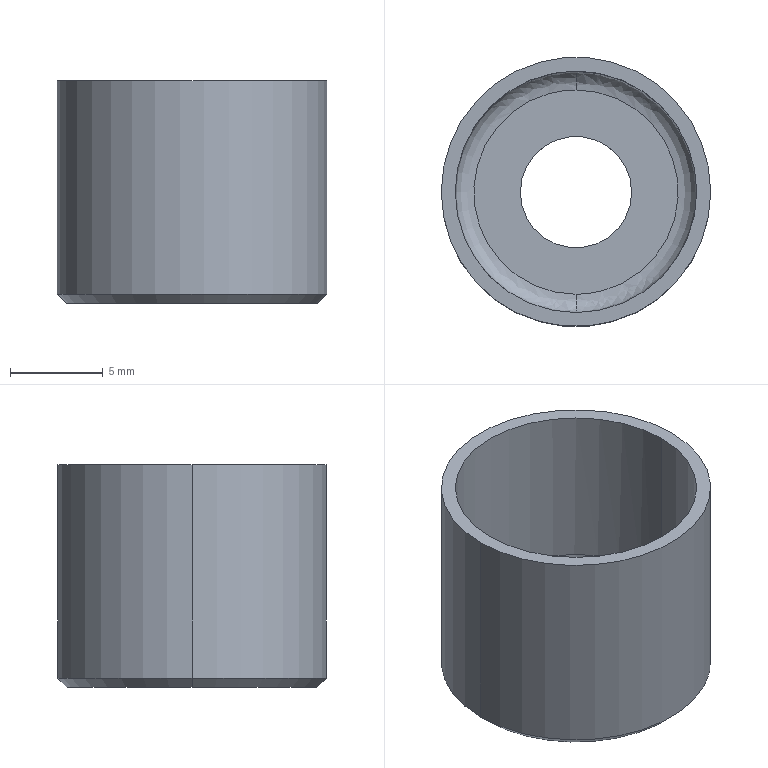Part | SolidWorks | features BaseBody 1 | 1 solid | 13 faces | box 14.5 x 14.5 x 12 mm | volume 600.582 mm3 | cylinder 6 | plane 3 | spline 2 | cone 2 | commonest cylinder face diameters 6 x2 13 x2 14.5 x2
STEP:
#1=CARTESIAN_POINT('',(480.537,43.215,-64.134));
#2=VERTEX_POINT('',#1);
#3=CARTESIAN_POINT('',(480.537,32.215,-64.134));
#4=VERTEX_POINT('',#3);
#5=CARTESIAN_POINT('',(480.537,43.215,-64.134));
#6=CARTESIAN_POINT('',(491.537,43.215,-64.134));
#7=CARTESIAN_POINT('',(491.537,32.215,-64.134));
#8=CARTESIAN_POINT('',(480.537,32.215,-64.134));
#9=(BOUNDED_CURVE()B_SPLINE_CURVE(3,(#5,#6,#7,#8),.UNSPECIFIED.,.F.,.F.)B_SPLINE_CURVE_WITH_KNOTS((4,4),(0.,1.),.UNSPECIFIED.)CURVE()GEOMETRIC_REPRESENTATION_ITEM()RATIONAL_B_SPLINE_CURVE((1.,0.3333,0.3333,1.))REPRESENTATION_ITEM(''));
#10=EDGE_CURVE('',#2,#4,#9,.T.);
#11=ORIENTED_EDGE('',*,*,#10,.T.);
#12=CARTESIAN_POINT('',(480.537,31.215,-63.134));
#13=VERTEX_POINT('',#12);
#14=CARTESIAN_POINT('',(480.537,32.215,-64.134));
#15=CARTESIAN_POINT('',(480.537,32.089,-64.134));
#16=CARTESIAN_POINT('',(480.537,31.827,-64.084));
#17=CARTESIAN_POINT('',(480.537,31.488,-63.861));
#18=CARTESIAN_POINT('',(480.537,31.265,-63.521));
#19=CARTESIAN_POINT('',(480.537,31.215,-63.26));
#20=CARTESIAN_POINT('',(480.537,31.215,-63.134));
#21=B_SPLINE_CURVE_WITH_KNOTS('',3,(#14,#15,#16,#17,#18,#19,#20),.UNSPECIFIED.,.F.,.F.,(4,1,1,1,4),(0.01923,0.25,0.5,0.75,0.9808),.UNSPECIFIED.);
#22=EDGE_CURVE('',#4,#13,#21,.T.);
#23=ORIENTED_EDGE('',*,*,#22,.T.);
#24=CARTESIAN_POINT('',(487.037,37.715,-63.134));
#25=VERTEX_POINT('',#24);
#26=CARTESIAN_POINT('',(487.037,37.715,-63.134));
#27=CARTESIAN_POINT('',(487.037,36.864,-63.134));
#28=CARTESIAN_POINT('',(486.868,36.013,-63.134));
#29=CARTESIAN_POINT('',(486.216,34.441,-63.134));
#30=CARTESIAN_POINT('',(485.735,33.72,-63.134));
#31=CARTESIAN_POINT('',(484.531,32.517,-63.134));
#32=CARTESIAN_POINT('',(483.81,32.035,-63.134));
#33=CARTESIAN_POINT('',(482.238,31.384,-63.134));
#34=CARTESIAN_POINT('',(481.388,31.215,-63.134));
#35=CARTESIAN_POINT('',(480.537,31.215,-63.134));
#36=B_SPLINE_CURVE_WITH_KNOTS('',3,(#26,#27,#28,#29,#30,#31,#32,#33,#34,#35),.UNSPECIFIED.,.F.,.F.,(4,2,2,2,4),(0.5,0.625,0.75,0.875,1.),.UNSPECIFIED.);
#37=EDGE_CURVE('',#25,#13,#36,.T.);
#38=ORIENTED_EDGE('',*,*,#37,.F.);
#39=CARTESIAN_POINT('',(480.537,44.215,-63.134));
#40=VERTEX_POINT('',#39);
#41=CARTESIAN_POINT('',(480.537,44.215,-63.134));
#42=CARTESIAN_POINT('',(481.388,44.215,-63.134));
#43=CARTESIAN_POINT('',(482.238,44.046,-63.134));
#44=CARTESIAN_POINT('',(483.81,43.394,-63.134));
#45=CARTESIAN_POINT('',(484.531,42.913,-63.134));
#46=CARTESIAN_POINT('',(485.735,41.709,-63.134));
#47=CARTESIAN_POINT('',(486.216,40.988,-63.134));
#48=CARTESIAN_POINT('',(486.868,39.416,-63.134));
#49=CARTESIAN_POINT('',(487.037,38.566,-63.134));
#50=CARTESIAN_POINT('',(487.037,37.715,-63.134));
#51=B_SPLINE_CURVE_WITH_KNOTS('',3,(#41,#42,#43,#44,#45,#46,#47,#48,#49,#50),.UNSPECIFIED.,.F.,.F.,(4,2,2,2,4),(0.,0.125,0.25,0.375,0.5),.UNSPECIFIED.);
#52=EDGE_CURVE('',#40,#25,#51,.T.);
#53=ORIENTED_EDGE('',*,*,#52,.F.);
#54=CARTESIAN_POINT('',(480.537,43.215,-64.134));
#55=CARTESIAN_POINT('',(480.537,43.34,-64.134));
#56=CARTESIAN_POINT('',(480.537,43.602,-64.084));
#57=CARTESIAN_POINT('',(480.537,43.942,-63.861));
#58=CARTESIAN_POINT('',(480.537,44.165,-63.521));
#59=CARTESIAN_POINT('',(480.537,44.215,-63.26));
#60=CARTESIAN_POINT('',(480.537,44.215,-63.134));
#61=B_SPLINE_CURVE_WITH_KNOTS('',3,(#54,#55,#56,#57,#58,#59,#60),.UNSPECIFIED.,.F.,.F.,(4,1,1,1,4),(0.01923,0.25,0.5,0.75,0.9808),.UNSPECIFIED.);
#62=EDGE_CURVE('',#2,#40,#61,.T.);
#63=ORIENTED_EDGE('',*,*,#62,.F.);
#64=EDGE_LOOP('',(#11,#23,#38,#53,#63));
#65=FACE_OUTER_BOUND('',#64,.T.);
#66=CARTESIAN_POINT('',(480.537,32.215,-64.134));
#67=CARTESIAN_POINT('',(491.537,32.215,-64.134));
#68=CARTESIAN_POINT('',(491.537,43.215,-64.134));
#69=CARTESIAN_POINT('',(480.537,43.215,-64.134));
#70=CARTESIAN_POINT('',(480.537,32.089,-64.134));
#71=CARTESIAN_POINT('',(491.788,32.089,-64.134));
#72=CARTESIAN_POINT('',(491.788,43.34,-64.134));
#73=CARTESIAN_POINT('',(480.537,43.34,-64.134));
#74=CARTESIAN_POINT('',(480.537,31.827,-64.084));
#75=CARTESIAN_POINT('',(492.312,31.827,-64.084));
#76=CARTESIAN_POINT('',(492.312,43.602,-64.084));
#77=CARTESIAN_POINT('',(480.537,43.602,-64.084));
#78=CARTESIAN_POINT('',(480.537,31.488,-63.861));
#79=CARTESIAN_POINT('',(492.991,31.488,-63.861));
#80=CARTESIAN_POINT('',(492.991,43.942,-63.861));
#81=CARTESIAN_POINT('',(480.537,43.942,-63.861));
#82=CARTESIAN_POINT('',(480.537,31.265,-63.521));
#83=CARTESIAN_POINT('',(493.437,31.265,-63.521));
#84=CARTESIAN_POINT('',(493.437,44.165,-63.521));
#85=CARTESIAN_POINT('',(480.537,44.165,-63.521));
#86=CARTESIAN_POINT('',(480.537,31.215,-63.26));
#87=CARTESIAN_POINT('',(493.537,31.215,-63.26));
#88=CARTESIAN_POINT('',(493.537,44.215,-63.26));
#89=CARTESIAN_POINT('',(480.537,44.215,-63.26));
#90=CARTESIAN_POINT('',(480.537,31.215,-63.134));
#91=CARTESIAN_POINT('',(493.537,31.215,-63.134));
#92=CARTESIAN_POINT('',(493.537,44.215,-63.134));
#93=CARTESIAN_POINT('',(480.537,44.215,-63.134));
#94=(BOUNDED_SURFACE()B_SPLINE_SURFACE(3,3,((#66,#67,#68,#69),(#70,#71,#72,#73),(#74,#75,#76,#77),(#78,#79,#80,#81),(#82,#83,#84,#85),(#86,#87,#88,#89),(#90,#91,#92,#93)),.UNSPECIFIED.,.F.,.F.,.F.)B_SPLINE_SURFACE_WITH_KNOTS((4,1,1,1,4),(4,4),(0.01923,0.25,0.5,0.75,0.9808),(0.,1.),.UNSPECIFIED.)GEOMETRIC_REPRESENTATION_ITEM()RATIONAL_B_SPLINE_SURFACE(((1.,0.3333,0.3333,1.),(1.,0.3333,0.3333,1.),(1.,0.3333,0.3333,1.),(1.,0.3333,0.3333,1.),(1.,0.3333,0.3333,1.),(1.,0.3333,0.3333,1.),(1.,0.3333,0.3333,1.)))REPRESENTATION_ITEM('')SURFACE());
#95=ADVANCED_FACE('',(#65),#94,.T.);
#96=CARTESIAN_POINT('',(473.287,37.715,-65.634));
#97=VERTEX_POINT('',#96);
#98=CARTESIAN_POINT('',(487.787,37.715,-65.634));
#99=VERTEX_POINT('',#98);
#100=CARTESIAN_POINT('',(480.537,37.715,-65.634));
#101=DIRECTION('',(0.000000013,0.,-1.));
#102=DIRECTION('',(0.,1.,0.));
#103=AXIS2_PLACEMENT_3D('',#100,#101,#102);
#104=CIRCLE('',#103,7.25);
#105=EDGE_CURVE('',#97,#99,#104,.T.);
#106=ORIENTED_EDGE('',*,*,#105,.F.);
#107=CARTESIAN_POINT('',(473.287,37.715,-54.134));
#108=VERTEX_POINT('',#107);
#109=CARTESIAN_POINT('',(473.287,37.715,-65.634));
#110=DIRECTION('',(-0.000000013,0.,1.));
#111=VECTOR('',#110,1000.);
#112=LINE('',#109,#111);
#113=EDGE_CURVE('',#97,#108,#112,.T.);
#114=ORIENTED_EDGE('',*,*,#113,.T.);
#115=CARTESIAN_POINT('',(487.787,37.715,-54.134));
#116=VERTEX_POINT('',#115);
#117=CARTESIAN_POINT('',(480.537,37.715,-54.134));
#118=DIRECTION('',(-0.000000013,0.,1.));
#119=DIRECTION('',(1.,0.,0.000000013));
#120=AXIS2_PLACEMENT_3D('',#117,#118,#119);
#121=CIRCLE('',#120,7.25);
#122=EDGE_CURVE('',#116,#108,#121,.T.);
#123=ORIENTED_EDGE('',*,*,#122,.F.);
#124=CARTESIAN_POINT('',(487.787,37.715,-65.634));
#125=DIRECTION('',(-0.000000013,0.,1.));
#126=VECTOR('',#125,1000.);
#127=LINE('',#124,#126);
#128=EDGE_CURVE('',#99,#116,#127,.T.);
#129=ORIENTED_EDGE('',*,*,#128,.F.);
#130=EDGE_LOOP('',(#106,#114,#123,#129));
#131=FACE_OUTER_BOUND('',#130,.T.);
#132=CARTESIAN_POINT('',(480.537,37.715,-65.634));
#133=DIRECTION('',(-0.000000013,0.,1.));
#134=DIRECTION('',(1.,0.,0.000000013));
#135=AXIS2_PLACEMENT_3D('',#132,#133,#134);
#136=CYLINDRICAL_SURFACE('',#135,7.25);
#137=ADVANCED_FACE('',(#131),#136,.T.);
#138=CARTESIAN_POINT('',(473.787,37.715,-66.134));
#139=VERTEX_POINT('',#138);
#140=CARTESIAN_POINT('',(487.287,37.715,-66.134));
#141=VERTEX_POINT('',#140);
#142=CARTESIAN_POINT('',(480.537,37.715,-66.134));
#143=DIRECTION('',(0.000000013,0.,-1.));
#144=DIRECTION('',(1.,0.,0.000000013));
#145=AXIS2_PLACEMENT_3D('',#142,#143,#144);
#146=CIRCLE('',#145,6.75);
#147=EDGE_CURVE('',#139,#141,#146,.T.);
#148=ORIENTED_EDGE('',*,*,#147,.F.);
#149=CARTESIAN_POINT('',(473.787,37.715,-66.134));
#150=DIRECTION('',(-0.7071,0.,0.7071));
#151=VECTOR('',#150,1000.);
#152=LINE('',#149,#151);
#153=EDGE_CURVE('',#139,#97,#152,.T.);
#154=ORIENTED_EDGE('',*,*,#153,.T.);
#155=ORIENTED_EDGE('',*,*,#105,.T.);
#156=CARTESIAN_POINT('',(487.287,37.715,-66.134));
#157=DIRECTION('',(0.7071,0.,0.7071));
#158=VECTOR('',#157,1000.);
#159=LINE('',#156,#158);
#160=EDGE_CURVE('',#141,#99,#159,.T.);
#161=ORIENTED_EDGE('',*,*,#160,.F.);
#162=EDGE_LOOP('',(#148,#154,#155,#161));
#163=FACE_OUTER_BOUND('',#162,.T.);
#164=CARTESIAN_POINT('',(480.537,37.715,-66.134));
#165=DIRECTION('',(-0.000000013,0.,1.));
#166=DIRECTION('',(1.,0.,0.000000013));
#167=AXIS2_PLACEMENT_3D('',#164,#165,#166);
#168=CONICAL_SURFACE('',#167,6.75,0.7854);
#169=ADVANCED_FACE('',(#163),#168,.T.);
#170=CARTESIAN_POINT('',(474.037,37.715,-63.134));
#171=VERTEX_POINT('',#170);
#172=CARTESIAN_POINT('',(480.537,31.215,-63.134));
#173=CARTESIAN_POINT('',(479.686,31.215,-63.134));
#174=CARTESIAN_POINT('',(478.835,31.384,-63.134));
#175=CARTESIAN_POINT('',(477.263,32.035,-63.134));
#176=CARTESIAN_POINT('',(476.542,32.517,-63.134));
#177=CARTESIAN_POINT('',(475.339,33.72,-63.134));
#178=CARTESIAN_POINT('',(474.857,34.441,-63.134));
#179=CARTESIAN_POINT('',(474.206,36.013,-63.134));
#180=CARTESIAN_POINT('',(474.037,36.864,-63.134));
#181=CARTESIAN_POINT('',(474.037,37.715,-63.134));
#182=B_SPLINE_CURVE_WITH_KNOTS('',3,(#172,#173,#174,#175,#176,#177,#178,#179,#180,#181),.UNSPECIFIED.,.F.,.F.,(4,2,2,2,4),(0.,0.125,0.25,0.375,0.5),.UNSPECIFIED.);
#183=EDGE_CURVE('',#13,#171,#182,.T.);
#184=ORIENTED_EDGE('',*,*,#183,.T.);
#185=CARTESIAN_POINT('',(474.037,37.715,-54.134));
#186=VERTEX_POINT('',#185);
#187=CARTESIAN_POINT('',(474.037,37.715,-63.134));
#188=DIRECTION('',(-0.000000013,0.,1.));
#189=VECTOR('',#188,1000.);
#190=LINE('',#187,#189);
#191=EDGE_CURVE('',#171,#186,#190,.T.);
#192=ORIENTED_EDGE('',*,*,#191,.T.);
#193=CARTESIAN_POINT('',(487.037,37.715,-54.134));
#194=VERTEX_POINT('',#193);
#195=CARTESIAN_POINT('',(480.537,37.715,-54.134));
#196=DIRECTION('',(0.000000013,0.,-1.));
#197=DIRECTION('',(1.,0.,0.000000013));
#198=AXIS2_PLACEMENT_3D('',#195,#196,#197);
#199=CIRCLE('',#198,6.5);
#200=EDGE_CURVE('',#194,#186,#199,.T.);
#201=ORIENTED_EDGE('',*,*,#200,.F.);
#202=CARTESIAN_POINT('',(487.037,37.715,-63.134));
#203=DIRECTION('',(-0.000000013,0.,1.));
#204=VECTOR('',#203,1000.);
#205=LINE('',#202,#204);
#206=EDGE_CURVE('',#25,#194,#205,.T.);
#207=ORIENTED_EDGE('',*,*,#206,.F.);
#208=ORIENTED_EDGE('',*,*,#37,.T.);
#209=EDGE_LOOP('',(#184,#192,#201,#207,#208));
#210=FACE_OUTER_BOUND('',#209,.T.);
#211=CARTESIAN_POINT('',(480.537,37.715,-63.134));
#212=DIRECTION('',(-0.000000013,0.,1.));
#213=DIRECTION('',(1.,0.,0.000000013));
#214=AXIS2_PLACEMENT_3D('',#211,#212,#213);
#215=CYLINDRICAL_SURFACE('',#214,6.5);
#216=ADVANCED_FACE('',(#210),#215,.F.);
#217=CARTESIAN_POINT('',(483.537,37.715,-66.134));
#218=VERTEX_POINT('',#217);
#219=CARTESIAN_POINT('',(477.537,37.715,-66.134));
#220=VERTEX_POINT('',#219);
#221=CARTESIAN_POINT('',(480.537,37.715,-66.134));
#222=DIRECTION('',(0.000000013,0.,-1.));
#223=DIRECTION('',(1.,0.,0.000000013));
#224=AXIS2_PLACEMENT_3D('',#221,#222,#223);
#225=CIRCLE('',#224,3.);
#226=EDGE_CURVE('',#218,#220,#225,.T.);
#227=ORIENTED_EDGE('',*,*,#226,.T.);
#228=CARTESIAN_POINT('',(477.537,37.715,-64.134));
#229=VERTEX_POINT('',#228);
#230=CARTESIAN_POINT('',(477.537,37.715,-66.134));
#231=DIRECTION('',(-0.000000013,0.,1.));
#232=VECTOR('',#231,1000.);
#233=LINE('',#230,#232);
#234=EDGE_CURVE('',#220,#229,#233,.T.);
#235=ORIENTED_EDGE('',*,*,#234,.T.);
#236=CARTESIAN_POINT('',(483.537,37.715,-64.134));
#237=VERTEX_POINT('',#236);
#238=CARTESIAN_POINT('',(480.537,37.715,-64.134));
#239=DIRECTION('',(-0.000000013,0.,1.));
#240=DIRECTION('',(1.,0.,0.000000013));
#241=AXIS2_PLACEMENT_3D('',#238,#239,#240);
#242=CIRCLE('',#241,3.);
#243=EDGE_CURVE('',#229,#237,#242,.T.);
#244=ORIENTED_EDGE('',*,*,#243,.T.);
#245=CARTESIAN_POINT('',(483.537,37.715,-66.134));
#246=DIRECTION('',(-0.000000013,0.,1.));
#247=VECTOR('',#246,1000.);
#248=LINE('',#245,#247);
#249=EDGE_CURVE('',#218,#237,#248,.T.);
#250=ORIENTED_EDGE('',*,*,#249,.F.);
#251=EDGE_LOOP('',(#227,#235,#244,#250));
#252=FACE_OUTER_BOUND('',#251,.T.);
#253=CARTESIAN_POINT('',(480.537,37.715,-66.134));
#254=DIRECTION('',(-0.000000013,0.,1.));
#255=DIRECTION('',(1.,0.,0.000000013));
#256=AXIS2_PLACEMENT_3D('',#253,#254,#255);
#257=CYLINDRICAL_SURFACE('',#256,3.);
#258=ADVANCED_FACE('',(#252),#257,.F.);
#259=ORIENTED_EDGE('',*,*,#113,.F.);
#260=CARTESIAN_POINT('',(480.537,37.715,-65.634));
#261=DIRECTION('',(0.000000013,0.,-1.));
#262=DIRECTION('',(0.,1.,0.));
#263=AXIS2_PLACEMENT_3D('',#260,#261,#262);
#264=CIRCLE('',#263,7.25);
#265=EDGE_CURVE('',#99,#97,#264,.T.);
#266=ORIENTED_EDGE('',*,*,#265,.F.);
#267=ORIENTED_EDGE('',*,*,#128,.T.);
#268=CARTESIAN_POINT('',(480.537,37.715,-54.134));
#269=DIRECTION('',(-0.000000013,0.,1.));
#270=DIRECTION('',(1.,0.,0.000000013));
#271=AXIS2_PLACEMENT_3D('',#268,#269,#270);
#272=CIRCLE('',#271,7.25);
#273=EDGE_CURVE('',#108,#116,#272,.T.);
#274=ORIENTED_EDGE('',*,*,#273,.F.);
#275=EDGE_LOOP('',(#259,#266,#267,#274));
#276=FACE_OUTER_BOUND('',#275,.T.);
#277=CARTESIAN_POINT('',(480.537,37.715,-65.634));
#278=DIRECTION('',(-0.000000013,0.,1.));
#279=DIRECTION('',(1.,0.,0.000000013));
#280=AXIS2_PLACEMENT_3D('',#277,#278,#279);
#281=CYLINDRICAL_SURFACE('',#280,7.25);
#282=ADVANCED_FACE('',(#276),#281,.T.);
#283=ORIENTED_EDGE('',*,*,#153,.F.);
#284=CARTESIAN_POINT('',(480.537,37.715,-66.134));
#285=DIRECTION('',(0.000000013,0.,-1.));
#286=DIRECTION('',(1.,0.,0.000000013));
#287=AXIS2_PLACEMENT_3D('',#284,#285,#286);
#288=CIRCLE('',#287,6.75);
#289=EDGE_CURVE('',#141,#139,#288,.T.);
#290=ORIENTED_EDGE('',*,*,#289,.F.);
#291=ORIENTED_EDGE('',*,*,#160,.T.);
#292=ORIENTED_EDGE('',*,*,#265,.T.);
#293=EDGE_LOOP('',(#283,#290,#291,#292));
#294=FACE_OUTER_BOUND('',#293,.T.);
#295=CARTESIAN_POINT('',(480.537,37.715,-66.134));
#296=DIRECTION('',(-0.000000013,0.,1.));
#297=DIRECTION('',(1.,0.,0.000000013));
#298=AXIS2_PLACEMENT_3D('',#295,#296,#297);
#299=CONICAL_SURFACE('',#298,6.75,0.7854);
#300=ADVANCED_FACE('',(#294),#299,.T.);
#301=ORIENTED_EDGE('',*,*,#200,.T.);
#302=CARTESIAN_POINT('',(480.537,37.715,-54.134));
#303=DIRECTION('',(0.000000013,0.,-1.));
#304=DIRECTION('',(1.,0.,0.000000013));
#305=AXIS2_PLACEMENT_3D('',#302,#303,#304);
#306=CIRCLE('',#305,6.5);
#307=EDGE_CURVE('',#186,#194,#306,.T.);
#308=ORIENTED_EDGE('',*,*,#307,.T.);
#309=EDGE_LOOP('',(#301,#308));
#310=FACE_BOUND('',#309,.T.);
#311=ORIENTED_EDGE('',*,*,#122,.T.);
#312=ORIENTED_EDGE('',*,*,#273,.T.);
#313=EDGE_LOOP('',(#311,#312));
#314=FACE_OUTER_BOUND('',#313,.T.);
#315=CARTESIAN_POINT('',(488.081,30.175,-54.134));
#316=DIRECTION('',(-0.000000013,0.,1.));
#317=DIRECTION('',(0.,1.,0.));
#318=AXIS2_PLACEMENT_3D('',#315,#316,#317);
#319=PLANE('',#318);
#320=ADVANCED_FACE('',(#310,#314),#319,.T.);
#321=ORIENTED_EDGE('',*,*,#226,.F.);
#322=CARTESIAN_POINT('',(480.537,37.715,-66.134));
#323=DIRECTION('',(0.000000013,0.,-1.));
#324=DIRECTION('',(1.,0.,0.000000013));
#325=AXIS2_PLACEMENT_3D('',#322,#323,#324);
#326=CIRCLE('',#325,3.);
#327=EDGE_CURVE('',#220,#218,#326,.T.);
#328=ORIENTED_EDGE('',*,*,#327,.F.);
#329=EDGE_LOOP('',(#321,#328));
#330=FACE_BOUND('',#329,.T.);
#331=ORIENTED_EDGE('',*,*,#289,.T.);
#332=ORIENTED_EDGE('',*,*,#147,.T.);
#333=EDGE_LOOP('',(#331,#332));
#334=FACE_OUTER_BOUND('',#333,.T.);
#335=CARTESIAN_POINT('',(487.563,30.695,-66.134));
#336=DIRECTION('',(-0.000000013,0.,1.));
#337=DIRECTION('',(0.,1.,0.));
#338=AXIS2_PLACEMENT_3D('',#335,#336,#337);
#339=PLANE('',#338);
#340=ADVANCED_FACE('',(#330,#334),#339,.F.);
#341=ORIENTED_EDGE('',*,*,#191,.F.);
#342=CARTESIAN_POINT('',(474.037,37.715,-63.134));
#343=CARTESIAN_POINT('',(474.037,38.566,-63.134));
#344=CARTESIAN_POINT('',(474.206,39.416,-63.134));
#345=CARTESIAN_POINT('',(474.857,40.988,-63.134));
#346=CARTESIAN_POINT('',(475.339,41.709,-63.134));
#347=CARTESIAN_POINT('',(476.542,42.913,-63.134));
#348=CARTESIAN_POINT('',(477.263,43.394,-63.134));
#349=CARTESIAN_POINT('',(478.835,44.046,-63.134));
#350=CARTESIAN_POINT('',(479.686,44.215,-63.134));
#351=CARTESIAN_POINT('',(480.537,44.215,-63.134));
#352=B_SPLINE_CURVE_WITH_KNOTS('',3,(#342,#343,#344,#345,#346,#347,#348,#349,#350,#351),.UNSPECIFIED.,.F.,.F.,(4,2,2,2,4),(0.5,0.625,0.75,0.875,1.),.UNSPECIFIED.);
#353=EDGE_CURVE('',#171,#40,#352,.T.);
#354=ORIENTED_EDGE('',*,*,#353,.T.);
#355=ORIENTED_EDGE('',*,*,#52,.T.);
#356=ORIENTED_EDGE('',*,*,#206,.T.);
#357=ORIENTED_EDGE('',*,*,#307,.F.);
#358=EDGE_LOOP('',(#341,#354,#355,#356,#357));
#359=FACE_OUTER_BOUND('',#358,.T.);
#360=CARTESIAN_POINT('',(480.537,37.715,-63.134));
#361=DIRECTION('',(-0.000000013,0.,1.));
#362=DIRECTION('',(1.,0.,0.000000013));
#363=AXIS2_PLACEMENT_3D('',#360,#361,#362);
#364=CYLINDRICAL_SURFACE('',#363,6.5);
#365=ADVANCED_FACE('',(#359),#364,.F.);
#366=ORIENTED_EDGE('',*,*,#234,.F.);
#367=ORIENTED_EDGE('',*,*,#327,.T.);
#368=ORIENTED_EDGE('',*,*,#249,.T.);
#369=CARTESIAN_POINT('',(480.537,37.715,-64.134));
#370=DIRECTION('',(-0.000000013,0.,1.));
#371=DIRECTION('',(1.,0.,0.000000013));
#372=AXIS2_PLACEMENT_3D('',#369,#370,#371);
#373=CIRCLE('',#372,3.);
#374=EDGE_CURVE('',#237,#229,#373,.T.);
#375=ORIENTED_EDGE('',*,*,#374,.T.);
#376=EDGE_LOOP('',(#366,#367,#368,#375));
#377=FACE_OUTER_BOUND('',#376,.T.);
#378=CARTESIAN_POINT('',(480.537,37.715,-66.134));
#379=DIRECTION('',(-0.000000013,0.,1.));
#380=DIRECTION('',(1.,0.,0.000000013));
#381=AXIS2_PLACEMENT_3D('',#378,#379,#380);
#382=CYLINDRICAL_SURFACE('',#381,3.);
#383=ADVANCED_FACE('',(#377),#382,.F.);
#384=ORIENTED_EDGE('',*,*,#22,.F.);
#385=CARTESIAN_POINT('',(480.537,32.215,-64.134));
#386=CARTESIAN_POINT('',(469.537,32.215,-64.134));
#387=CARTESIAN_POINT('',(469.537,43.215,-64.134));
#388=CARTESIAN_POINT('',(480.537,43.215,-64.134));
#389=(BOUNDED_CURVE()B_SPLINE_CURVE(3,(#385,#386,#387,#388),.UNSPECIFIED.,.F.,.F.)B_SPLINE_CURVE_WITH_KNOTS((4,4),(0.,1.),.UNSPECIFIED.)CURVE()GEOMETRIC_REPRESENTATION_ITEM()RATIONAL_B_SPLINE_CURVE((1.,0.3333,0.3333,1.))REPRESENTATION_ITEM(''));
#390=EDGE_CURVE('',#4,#2,#389,.T.);
#391=ORIENTED_EDGE('',*,*,#390,.T.);
#392=ORIENTED_EDGE('',*,*,#62,.T.);
#393=ORIENTED_EDGE('',*,*,#353,.F.);
#394=ORIENTED_EDGE('',*,*,#183,.F.);
#395=EDGE_LOOP('',(#384,#391,#392,#393,#394));
#396=FACE_OUTER_BOUND('',#395,.T.);
#397=CARTESIAN_POINT('',(480.537,43.215,-64.134));
#398=CARTESIAN_POINT('',(469.537,43.215,-64.134));
#399=CARTESIAN_POINT('',(469.537,32.215,-64.134));
#400=CARTESIAN_POINT('',(480.537,32.215,-64.134));
#401=CARTESIAN_POINT('',(480.537,43.34,-64.134));
#402=CARTESIAN_POINT('',(469.286,43.34,-64.134));
#403=CARTESIAN_POINT('',(469.286,32.089,-64.134));
#404=CARTESIAN_POINT('',(480.537,32.089,-64.134));
#405=CARTESIAN_POINT('',(480.537,43.602,-64.084));
#406=CARTESIAN_POINT('',(468.762,43.602,-64.084));
#407=CARTESIAN_POINT('',(468.762,31.827,-64.084));
#408=CARTESIAN_POINT('',(480.537,31.827,-64.084));
#409=CARTESIAN_POINT('',(480.537,43.942,-63.861));
#410=CARTESIAN_POINT('',(468.083,43.942,-63.861));
#411=CARTESIAN_POINT('',(468.083,31.488,-63.861));
#412=CARTESIAN_POINT('',(480.537,31.488,-63.861));
#413=CARTESIAN_POINT('',(480.537,44.165,-63.521));
#414=CARTESIAN_POINT('',(467.637,44.165,-63.521));
#415=CARTESIAN_POINT('',(467.637,31.265,-63.521));
#416=CARTESIAN_POINT('',(480.537,31.265,-63.521));
#417=CARTESIAN_POINT('',(480.537,44.215,-63.26));
#418=CARTESIAN_POINT('',(467.537,44.215,-63.26));
#419=CARTESIAN_POINT('',(467.537,31.215,-63.26));
#420=CARTESIAN_POINT('',(480.537,31.215,-63.26));
#421=CARTESIAN_POINT('',(480.537,44.215,-63.134));
#422=CARTESIAN_POINT('',(467.537,44.215,-63.134));
#423=CARTESIAN_POINT('',(467.537,31.215,-63.134));
#424=CARTESIAN_POINT('',(480.537,31.215,-63.134));
#425=(BOUNDED_SURFACE()B_SPLINE_SURFACE(3,3,((#397,#398,#399,#400),(#401,#402,#403,#404),(#405,#406,#407,#408),(#409,#410,#411,#412),(#413,#414,#415,#416),(#417,#418,#419,#420),(#421,#422,#423,#424)),.UNSPECIFIED.,.F.,.F.,.F.)B_SPLINE_SURFACE_WITH_KNOTS((4,1,1,1,4),(4,4),(0.01923,0.25,0.5,0.75,0.9808),(0.,1.),.UNSPECIFIED.)GEOMETRIC_REPRESENTATION_ITEM()RATIONAL_B_SPLINE_SURFACE(((1.,0.3333,0.3333,1.),(1.,0.3333,0.3333,1.),(1.,0.3333,0.3333,1.),(1.,0.3333,0.3333,1.),(1.,0.3333,0.3333,1.),(1.,0.3333,0.3333,1.),(1.,0.3333,0.3333,1.)))REPRESENTATION_ITEM('')SURFACE());
#426=ADVANCED_FACE('',(#396),#425,.T.);
#427=ORIENTED_EDGE('',*,*,#374,.F.);
#428=ORIENTED_EDGE('',*,*,#243,.F.);
#429=EDGE_LOOP('',(#427,#428));
#430=FACE_BOUND('',#429,.T.);
#431=ORIENTED_EDGE('',*,*,#10,.F.);
#432=ORIENTED_EDGE('',*,*,#390,.F.);
#433=EDGE_LOOP('',(#431,#432));
#434=FACE_OUTER_BOUND('',#433,.T.);
#435=CARTESIAN_POINT('',(486.257,31.995,-64.134));
#436=DIRECTION('',(-0.000000013,0.,1.));
#437=DIRECTION('',(0.,1.,0.));
#438=AXIS2_PLACEMENT_3D('',#435,#436,#437);
#439=PLANE('',#438);
#440=ADVANCED_FACE('',(#430,#434),#439,.T.);
#441=CLOSED_SHELL('',(#95,#137,#169,#216,#258,#282,#300,#320,#340,#365,#383,#426,#440));
#442=MANIFOLD_SOLID_BREP('',#441);
#443=CARTESIAN_POINT('',(0.,0.,0.));
#444=DIRECTION('',(0.,0.,1.));
#445=DIRECTION('',(1.,0.,0.));
#446=AXIS2_PLACEMENT_3D('',#443,#444,#445);
#447=(LENGTH_UNIT()NAMED_UNIT(*)SI_UNIT(.MILLI.,.METRE.));
#448=UNCERTAINTY_MEASURE_WITH_UNIT(LENGTH_MEASURE(0.00001),#447,'','');
#449=(NAMED_UNIT(*)PLANE_ANGLE_UNIT()SI_UNIT($,.RADIAN.));
#450=(NAMED_UNIT(*)SI_UNIT($,.STERADIAN.)SOLID_ANGLE_UNIT());
#451=(GEOMETRIC_REPRESENTATION_CONTEXT(3)GLOBAL_UNCERTAINTY_ASSIGNED_CONTEXT((#448))GLOBAL_UNIT_ASSIGNED_CONTEXT((#447,#449,#450))REPRESENTATION_CONTEXT('',''));
#452=ADVANCED_BREP_SHAPE_REPRESENTATION('',(#442,#446),#451);